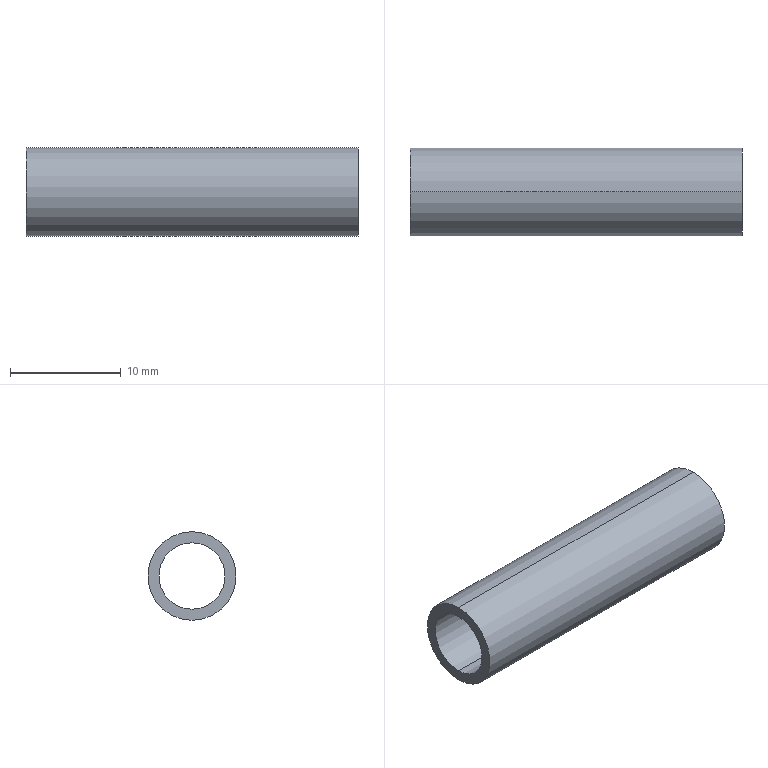Part | STEP file | 750078258 | 1 solid | 6 faces | box 30 x 8 x 8 mm | volume 659.734 mm3 | cylinder 4 | plane 2 | commonest cylinder face diameters 6 x2 8 x2
STEP:
#1=CARTESIAN_POINT('',(0.,0.,-4.));
#2=VERTEX_POINT('',#1);
#3=CARTESIAN_POINT('',(0.,0.,4.));
#4=VERTEX_POINT('',#3);
#5=CARTESIAN_POINT('',(0.,0.,0.));
#6=DIRECTION('',(1.,0.,0.));
#7=DIRECTION('',(0.,0.,-1.));
#8=AXIS2_PLACEMENT_3D('',#5,#6,#7);
#9=CIRCLE('',#8,4.);
#10=EDGE_CURVE('',#2,#4,#9,.T.);
#11=ORIENTED_EDGE('',*,*,#10,.T.);
#12=CARTESIAN_POINT('',(30.,0.,4.));
#13=VERTEX_POINT('',#12);
#14=CARTESIAN_POINT('',(0.,0.,4.));
#15=DIRECTION('',(1.,0.,0.));
#16=VECTOR('',#15,1000.);
#17=LINE('',#14,#16);
#18=EDGE_CURVE('',#4,#13,#17,.T.);
#19=ORIENTED_EDGE('',*,*,#18,.T.);
#20=CARTESIAN_POINT('',(30.,0.,-4.));
#21=VERTEX_POINT('',#20);
#22=CARTESIAN_POINT('',(30.,0.,0.));
#23=DIRECTION('',(-1.,0.,0.));
#24=DIRECTION('',(0.,0.,-1.));
#25=AXIS2_PLACEMENT_3D('',#22,#23,#24);
#26=CIRCLE('',#25,4.);
#27=EDGE_CURVE('',#13,#21,#26,.T.);
#28=ORIENTED_EDGE('',*,*,#27,.T.);
#29=CARTESIAN_POINT('',(0.,0.,-4.));
#30=DIRECTION('',(1.,0.,0.));
#31=VECTOR('',#30,1000.);
#32=LINE('',#29,#31);
#33=EDGE_CURVE('',#2,#21,#32,.T.);
#34=ORIENTED_EDGE('',*,*,#33,.F.);
#35=EDGE_LOOP('',(#11,#19,#28,#34));
#36=FACE_OUTER_BOUND('',#35,.T.);
#37=CARTESIAN_POINT('',(0.,0.,0.));
#38=DIRECTION('',(1.,0.,0.));
#39=DIRECTION('',(0.,0.,-1.));
#40=AXIS2_PLACEMENT_3D('',#37,#38,#39);
#41=CYLINDRICAL_SURFACE('',#40,4.);
#42=ADVANCED_FACE('',(#36),#41,.T.);
#43=CARTESIAN_POINT('',(0.,0.,3.));
#44=VERTEX_POINT('',#43);
#45=CARTESIAN_POINT('',(0.,0.,-3.));
#46=VERTEX_POINT('',#45);
#47=CARTESIAN_POINT('',(0.,0.,0.));
#48=DIRECTION('',(1.,0.,0.));
#49=DIRECTION('',(0.,0.,-1.));
#50=AXIS2_PLACEMENT_3D('',#47,#48,#49);
#51=CIRCLE('',#50,3.);
#52=EDGE_CURVE('',#44,#46,#51,.T.);
#53=ORIENTED_EDGE('',*,*,#52,.F.);
#54=CARTESIAN_POINT('',(30.,0.,3.));
#55=VERTEX_POINT('',#54);
#56=CARTESIAN_POINT('',(0.,0.,3.));
#57=DIRECTION('',(1.,0.,0.));
#58=VECTOR('',#57,1000.);
#59=LINE('',#56,#58);
#60=EDGE_CURVE('',#44,#55,#59,.T.);
#61=ORIENTED_EDGE('',*,*,#60,.T.);
#62=CARTESIAN_POINT('',(30.,0.,-3.));
#63=VERTEX_POINT('',#62);
#64=CARTESIAN_POINT('',(30.,0.,0.));
#65=DIRECTION('',(1.,0.,0.));
#66=DIRECTION('',(0.,0.,-1.));
#67=AXIS2_PLACEMENT_3D('',#64,#65,#66);
#68=CIRCLE('',#67,3.);
#69=EDGE_CURVE('',#55,#63,#68,.T.);
#70=ORIENTED_EDGE('',*,*,#69,.T.);
#71=CARTESIAN_POINT('',(0.,0.,-3.));
#72=DIRECTION('',(1.,0.,0.));
#73=VECTOR('',#72,1000.);
#74=LINE('',#71,#73);
#75=EDGE_CURVE('',#46,#63,#74,.T.);
#76=ORIENTED_EDGE('',*,*,#75,.F.);
#77=EDGE_LOOP('',(#53,#61,#70,#76));
#78=FACE_OUTER_BOUND('',#77,.T.);
#79=CARTESIAN_POINT('',(0.,0.,0.));
#80=DIRECTION('',(1.,0.,0.));
#81=DIRECTION('',(0.,0.,-1.));
#82=AXIS2_PLACEMENT_3D('',#79,#80,#81);
#83=CYLINDRICAL_SURFACE('',#82,3.);
#84=ADVANCED_FACE('',(#78),#83,.F.);
#85=ORIENTED_EDGE('',*,*,#18,.F.);
#86=CARTESIAN_POINT('',(0.,0.,0.));
#87=DIRECTION('',(1.,0.,0.));
#88=DIRECTION('',(0.,0.,-1.));
#89=AXIS2_PLACEMENT_3D('',#86,#87,#88);
#90=CIRCLE('',#89,4.);
#91=EDGE_CURVE('',#4,#2,#90,.T.);
#92=ORIENTED_EDGE('',*,*,#91,.T.);
#93=ORIENTED_EDGE('',*,*,#33,.T.);
#94=CARTESIAN_POINT('',(30.,0.,0.));
#95=DIRECTION('',(-1.,0.,0.));
#96=DIRECTION('',(0.,0.,-1.));
#97=AXIS2_PLACEMENT_3D('',#94,#95,#96);
#98=CIRCLE('',#97,4.);
#99=EDGE_CURVE('',#21,#13,#98,.T.);
#100=ORIENTED_EDGE('',*,*,#99,.T.);
#101=EDGE_LOOP('',(#85,#92,#93,#100));
#102=FACE_OUTER_BOUND('',#101,.T.);
#103=CARTESIAN_POINT('',(0.,0.,0.));
#104=DIRECTION('',(1.,0.,0.));
#105=DIRECTION('',(0.,0.,-1.));
#106=AXIS2_PLACEMENT_3D('',#103,#104,#105);
#107=CYLINDRICAL_SURFACE('',#106,4.);
#108=ADVANCED_FACE('',(#102),#107,.T.);
#109=ORIENTED_EDGE('',*,*,#99,.F.);
#110=ORIENTED_EDGE('',*,*,#27,.F.);
#111=EDGE_LOOP('',(#109,#110));
#112=FACE_OUTER_BOUND('',#111,.T.);
#113=CARTESIAN_POINT('',(30.,0.,0.));
#114=DIRECTION('',(1.,0.,0.));
#115=DIRECTION('',(0.,0.,-1.));
#116=AXIS2_PLACEMENT_3D('',#113,#114,#115);
#117=CIRCLE('',#116,3.);
#118=EDGE_CURVE('',#63,#55,#117,.T.);
#119=ORIENTED_EDGE('',*,*,#118,.F.);
#120=ORIENTED_EDGE('',*,*,#69,.F.);
#121=EDGE_LOOP('',(#119,#120));
#122=FACE_BOUND('',#121,.T.);
#123=CARTESIAN_POINT('',(30.,0.,0.));
#124=DIRECTION('',(-1.,0.,0.));
#125=DIRECTION('',(0.,0.,1.));
#126=AXIS2_PLACEMENT_3D('',#123,#124,#125);
#127=PLANE('',#126);
#128=ADVANCED_FACE('',(#112,#122),#127,.F.);
#129=ORIENTED_EDGE('',*,*,#10,.F.);
#130=ORIENTED_EDGE('',*,*,#91,.F.);
#131=EDGE_LOOP('',(#129,#130));
#132=FACE_OUTER_BOUND('',#131,.T.);
#133=CARTESIAN_POINT('',(0.,0.,0.));
#134=DIRECTION('',(1.,0.,0.));
#135=DIRECTION('',(0.,0.,-1.));
#136=AXIS2_PLACEMENT_3D('',#133,#134,#135);
#137=CIRCLE('',#136,3.);
#138=EDGE_CURVE('',#46,#44,#137,.T.);
#139=ORIENTED_EDGE('',*,*,#138,.T.);
#140=ORIENTED_EDGE('',*,*,#52,.T.);
#141=EDGE_LOOP('',(#139,#140));
#142=FACE_BOUND('',#141,.T.);
#143=CARTESIAN_POINT('',(0.,0.,0.));
#144=DIRECTION('',(-1.,0.,0.));
#145=DIRECTION('',(0.,0.,1.));
#146=AXIS2_PLACEMENT_3D('',#143,#144,#145);
#147=PLANE('',#146);
#148=ADVANCED_FACE('',(#132,#142),#147,.T.);
#149=ORIENTED_EDGE('',*,*,#60,.F.);
#150=ORIENTED_EDGE('',*,*,#138,.F.);
#151=ORIENTED_EDGE('',*,*,#75,.T.);
#152=ORIENTED_EDGE('',*,*,#118,.T.);
#153=EDGE_LOOP('',(#149,#150,#151,#152));
#154=FACE_OUTER_BOUND('',#153,.T.);
#155=CARTESIAN_POINT('',(0.,0.,0.));
#156=DIRECTION('',(1.,0.,0.));
#157=DIRECTION('',(0.,0.,-1.));
#158=AXIS2_PLACEMENT_3D('',#155,#156,#157);
#159=CYLINDRICAL_SURFACE('',#158,3.);
#160=ADVANCED_FACE('',(#154),#159,.F.);
#161=CLOSED_SHELL('',(#42,#84,#108,#128,#148,#160));
#162=MANIFOLD_SOLID_BREP('',#161);
#163=CARTESIAN_POINT('',(0.,0.,0.));
#164=DIRECTION('',(0.,0.,1.));
#165=DIRECTION('',(1.,0.,0.));
#166=AXIS2_PLACEMENT_3D('',#163,#164,#165);
#167=(LENGTH_UNIT()NAMED_UNIT(*)SI_UNIT(.MILLI.,.METRE.));
#168=UNCERTAINTY_MEASURE_WITH_UNIT(LENGTH_MEASURE(0.00001),#167,'','');
#169=(NAMED_UNIT(*)PLANE_ANGLE_UNIT()SI_UNIT($,.RADIAN.));
#170=(NAMED_UNIT(*)SI_UNIT($,.STERADIAN.)SOLID_ANGLE_UNIT());
#171=(GEOMETRIC_REPRESENTATION_CONTEXT(3)GLOBAL_UNCERTAINTY_ASSIGNED_CONTEXT((#168))GLOBAL_UNIT_ASSIGNED_CONTEXT((#167,#169,#170))REPRESENTATION_CONTEXT('',''));
#172=ADVANCED_BREP_SHAPE_REPRESENTATION('',(#162,#166),#171);